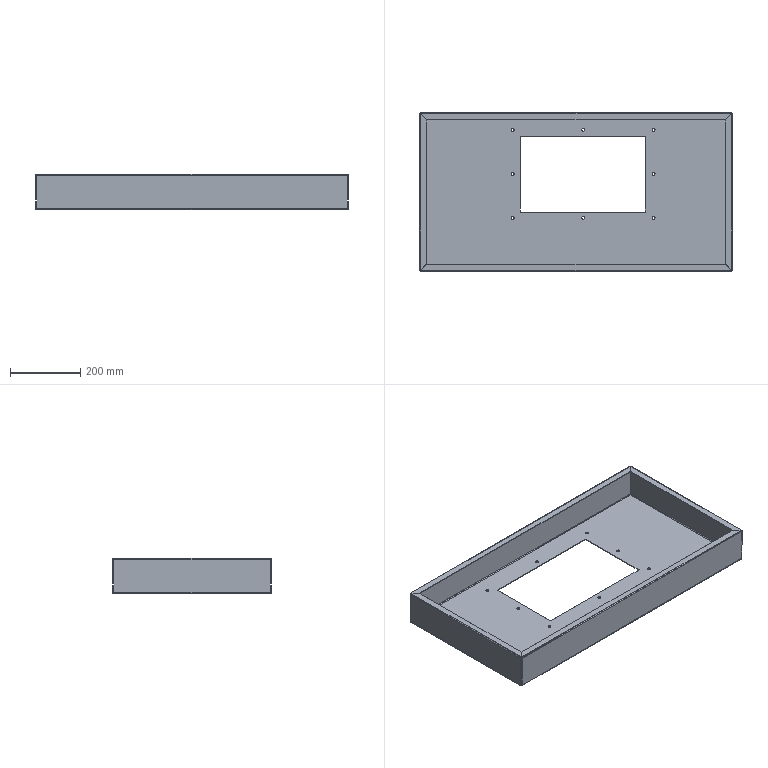Part | SolidWorks | features EdgeFlange 2, FlatPattern 1, SMBaseFlange 1, SheetMetal 1 | 1 solid | 90 faces | box 888 x 450 x 100 mm | volume 1248625 mm3 | plane 42 | cylinder 32 | spline 16 | commonest cylinder face diameters 8 x20 1.473 x4 4 x4 5.473 x4